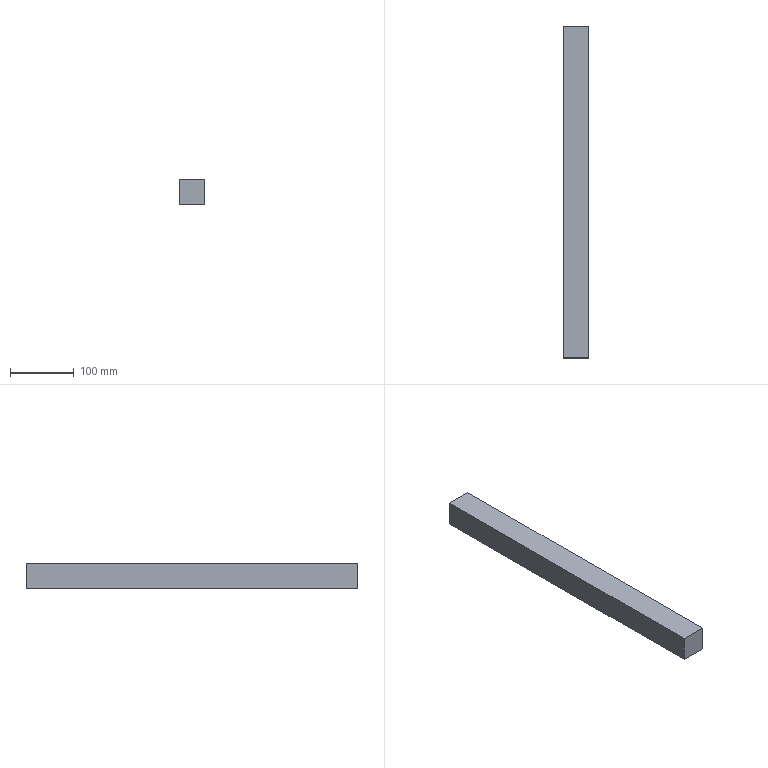Part | NX | features 凸台-拉伸25[3] 2 | 1 solid | 6 faces | box 40.475 x 520 x 40 mm | volume 841882 mm3 | plane 6
STEP:
#1=CARTESIAN_POINT('',(3973.,-40.,-402.985));
#2=VERTEX_POINT('',#1);
#3=CARTESIAN_POINT('',(3932.525,-40.,-402.985));
#4=VERTEX_POINT('',#3);
#5=CARTESIAN_POINT('',(3932.525,-40.,-402.985));
#6=DIRECTION('',(-1.,0.,0.));
#7=VECTOR('',#6,1000.);
#8=LINE('',#5,#7);
#9=EDGE_CURVE('',#2,#4,#8,.T.);
#10=ORIENTED_EDGE('',*,*,#9,.T.);
#11=CARTESIAN_POINT('',(3932.525,-40.,-362.985));
#12=VERTEX_POINT('',#11);
#13=CARTESIAN_POINT('',(3932.525,-40.,-402.985));
#14=DIRECTION('',(0.,0.,1.));
#15=VECTOR('',#14,1000.);
#16=LINE('',#13,#15);
#17=EDGE_CURVE('',#4,#12,#16,.T.);
#18=ORIENTED_EDGE('',*,*,#17,.T.);
#19=CARTESIAN_POINT('',(3973.,-40.,-362.985));
#20=VERTEX_POINT('',#19);
#21=CARTESIAN_POINT('',(3932.525,-40.,-362.985));
#22=DIRECTION('',(1.,0.,0.));
#23=VECTOR('',#22,1000.);
#24=LINE('',#21,#23);
#25=EDGE_CURVE('',#12,#20,#24,.T.);
#26=ORIENTED_EDGE('',*,*,#25,.T.);
#27=CARTESIAN_POINT('',(3973.,-40.,-402.985));
#28=DIRECTION('',(0.,0.,-1.));
#29=VECTOR('',#28,1000.);
#30=LINE('',#27,#29);
#31=EDGE_CURVE('',#20,#2,#30,.T.);
#32=ORIENTED_EDGE('',*,*,#31,.T.);
#33=EDGE_LOOP('',(#10,#18,#26,#32));
#34=FACE_BOUND('',#33,.T.);
#35=CARTESIAN_POINT('',(3933.,-40.,-1159.553));
#36=DIRECTION('',(0.,1.,0.));
#37=DIRECTION('',(-1.,0.,0.));
#38=AXIS2_PLACEMENT_3D('',#35,#36,#37);
#39=PLANE('',#38);
#40=ADVANCED_FACE('',(#34),#39,.T.);
#41=CARTESIAN_POINT('',(3932.525,-560.,-402.985));
#42=VERTEX_POINT('',#41);
#43=CARTESIAN_POINT('',(3932.525,-560.,-362.985));
#44=VERTEX_POINT('',#43);
#45=CARTESIAN_POINT('',(3932.525,-560.,-402.985));
#46=DIRECTION('',(0.,0.,1.));
#47=VECTOR('',#46,1000.);
#48=LINE('',#45,#47);
#49=EDGE_CURVE('',#42,#44,#48,.T.);
#50=ORIENTED_EDGE('',*,*,#49,.F.);
#51=CARTESIAN_POINT('',(3973.,-560.,-402.985));
#52=VERTEX_POINT('',#51);
#53=CARTESIAN_POINT('',(3932.525,-560.,-402.985));
#54=DIRECTION('',(-1.,0.,0.));
#55=VECTOR('',#54,1000.);
#56=LINE('',#53,#55);
#57=EDGE_CURVE('',#52,#42,#56,.T.);
#58=ORIENTED_EDGE('',*,*,#57,.F.);
#59=CARTESIAN_POINT('',(3973.,-560.,-362.985));
#60=VERTEX_POINT('',#59);
#61=CARTESIAN_POINT('',(3973.,-560.,-402.985));
#62=DIRECTION('',(0.,0.,-1.));
#63=VECTOR('',#62,1000.);
#64=LINE('',#61,#63);
#65=EDGE_CURVE('',#60,#52,#64,.T.);
#66=ORIENTED_EDGE('',*,*,#65,.F.);
#67=CARTESIAN_POINT('',(3932.525,-560.,-362.985));
#68=DIRECTION('',(1.,0.,0.));
#69=VECTOR('',#68,1000.);
#70=LINE('',#67,#69);
#71=EDGE_CURVE('',#44,#60,#70,.T.);
#72=ORIENTED_EDGE('',*,*,#71,.F.);
#73=EDGE_LOOP('',(#50,#58,#66,#72));
#74=FACE_BOUND('',#73,.T.);
#75=CARTESIAN_POINT('',(3000.,-560.,0.));
#76=DIRECTION('',(0.,1.,0.));
#77=DIRECTION('',(0.,0.,1.));
#78=AXIS2_PLACEMENT_3D('',#75,#76,#77);
#79=PLANE('',#78);
#80=ADVANCED_FACE('',(#74),#79,.F.);
#81=ORIENTED_EDGE('',*,*,#9,.F.);
#82=CARTESIAN_POINT('',(3973.,16.905,-402.985));
#83=DIRECTION('',(0.,-1.,0.));
#84=VECTOR('',#83,1000.);
#85=LINE('',#82,#84);
#86=EDGE_CURVE('',#2,#52,#85,.T.);
#87=ORIENTED_EDGE('',*,*,#86,.T.);
#88=ORIENTED_EDGE('',*,*,#57,.T.);
#89=CARTESIAN_POINT('',(3932.525,16.905,-402.985));
#90=DIRECTION('',(0.,-1.,0.));
#91=VECTOR('',#90,1000.);
#92=LINE('',#89,#91);
#93=EDGE_CURVE('',#4,#42,#92,.T.);
#94=ORIENTED_EDGE('',*,*,#93,.F.);
#95=EDGE_LOOP('',(#81,#87,#88,#94));
#96=FACE_BOUND('',#95,.T.);
#97=CARTESIAN_POINT('',(3932.525,16.905,-402.985));
#98=DIRECTION('',(0.,0.,1.));
#99=DIRECTION('',(1.,0.,0.));
#100=AXIS2_PLACEMENT_3D('',#97,#98,#99);
#101=PLANE('',#100);
#102=ADVANCED_FACE('',(#96),#101,.F.);
#103=ORIENTED_EDGE('',*,*,#31,.F.);
#104=CARTESIAN_POINT('',(3973.,16.905,-362.985));
#105=DIRECTION('',(0.,-1.,0.));
#106=VECTOR('',#105,1000.);
#107=LINE('',#104,#106);
#108=EDGE_CURVE('',#20,#60,#107,.T.);
#109=ORIENTED_EDGE('',*,*,#108,.T.);
#110=ORIENTED_EDGE('',*,*,#65,.T.);
#111=ORIENTED_EDGE('',*,*,#86,.F.);
#112=EDGE_LOOP('',(#103,#109,#110,#111));
#113=FACE_BOUND('',#112,.T.);
#114=CARTESIAN_POINT('',(3973.,16.905,-402.985));
#115=DIRECTION('',(-1.,0.,0.));
#116=DIRECTION('',(0.,0.,1.));
#117=AXIS2_PLACEMENT_3D('',#114,#115,#116);
#118=PLANE('',#117);
#119=ADVANCED_FACE('',(#113),#118,.F.);
#120=ORIENTED_EDGE('',*,*,#25,.F.);
#121=CARTESIAN_POINT('',(3932.525,16.905,-362.985));
#122=DIRECTION('',(0.,-1.,0.));
#123=VECTOR('',#122,1000.);
#124=LINE('',#121,#123);
#125=EDGE_CURVE('',#12,#44,#124,.T.);
#126=ORIENTED_EDGE('',*,*,#125,.T.);
#127=ORIENTED_EDGE('',*,*,#71,.T.);
#128=ORIENTED_EDGE('',*,*,#108,.F.);
#129=EDGE_LOOP('',(#120,#126,#127,#128));
#130=FACE_BOUND('',#129,.T.);
#131=CARTESIAN_POINT('',(3932.525,16.905,-362.985));
#132=DIRECTION('',(0.,0.,-1.));
#133=DIRECTION('',(-1.,0.,0.));
#134=AXIS2_PLACEMENT_3D('',#131,#132,#133);
#135=PLANE('',#134);
#136=ADVANCED_FACE('',(#130),#135,.F.);
#137=ORIENTED_EDGE('',*,*,#17,.F.);
#138=ORIENTED_EDGE('',*,*,#93,.T.);
#139=ORIENTED_EDGE('',*,*,#49,.T.);
#140=ORIENTED_EDGE('',*,*,#125,.F.);
#141=EDGE_LOOP('',(#137,#138,#139,#140));
#142=FACE_BOUND('',#141,.T.);
#143=CARTESIAN_POINT('',(3932.525,16.905,-402.985));
#144=DIRECTION('',(1.,0.,0.));
#145=DIRECTION('',(0.,0.,-1.));
#146=AXIS2_PLACEMENT_3D('',#143,#144,#145);
#147=PLANE('',#146);
#148=ADVANCED_FACE('',(#142),#147,.F.);
#149=CLOSED_SHELL('',(#40,#80,#102,#119,#136,#148));
#150=MANIFOLD_SOLID_BREP('',#149);
#151=(LENGTH_UNIT()NAMED_UNIT(*)SI_UNIT(.MILLI.,.METRE.));
#152=UNCERTAINTY_MEASURE_WITH_UNIT(LENGTH_MEASURE(0.00001),#151,'','');
#153=(NAMED_UNIT(*)PLANE_ANGLE_UNIT()SI_UNIT($,.RADIAN.));
#154=(NAMED_UNIT(*)SI_UNIT($,.STERADIAN.)SOLID_ANGLE_UNIT());
#155=(GEOMETRIC_REPRESENTATION_CONTEXT(3)GLOBAL_UNCERTAINTY_ASSIGNED_CONTEXT((#152))GLOBAL_UNIT_ASSIGNED_CONTEXT((#151,#153,#154))REPRESENTATION_CONTEXT('',''));
#156=ADVANCED_BREP_SHAPE_REPRESENTATION('',(#150),#155);